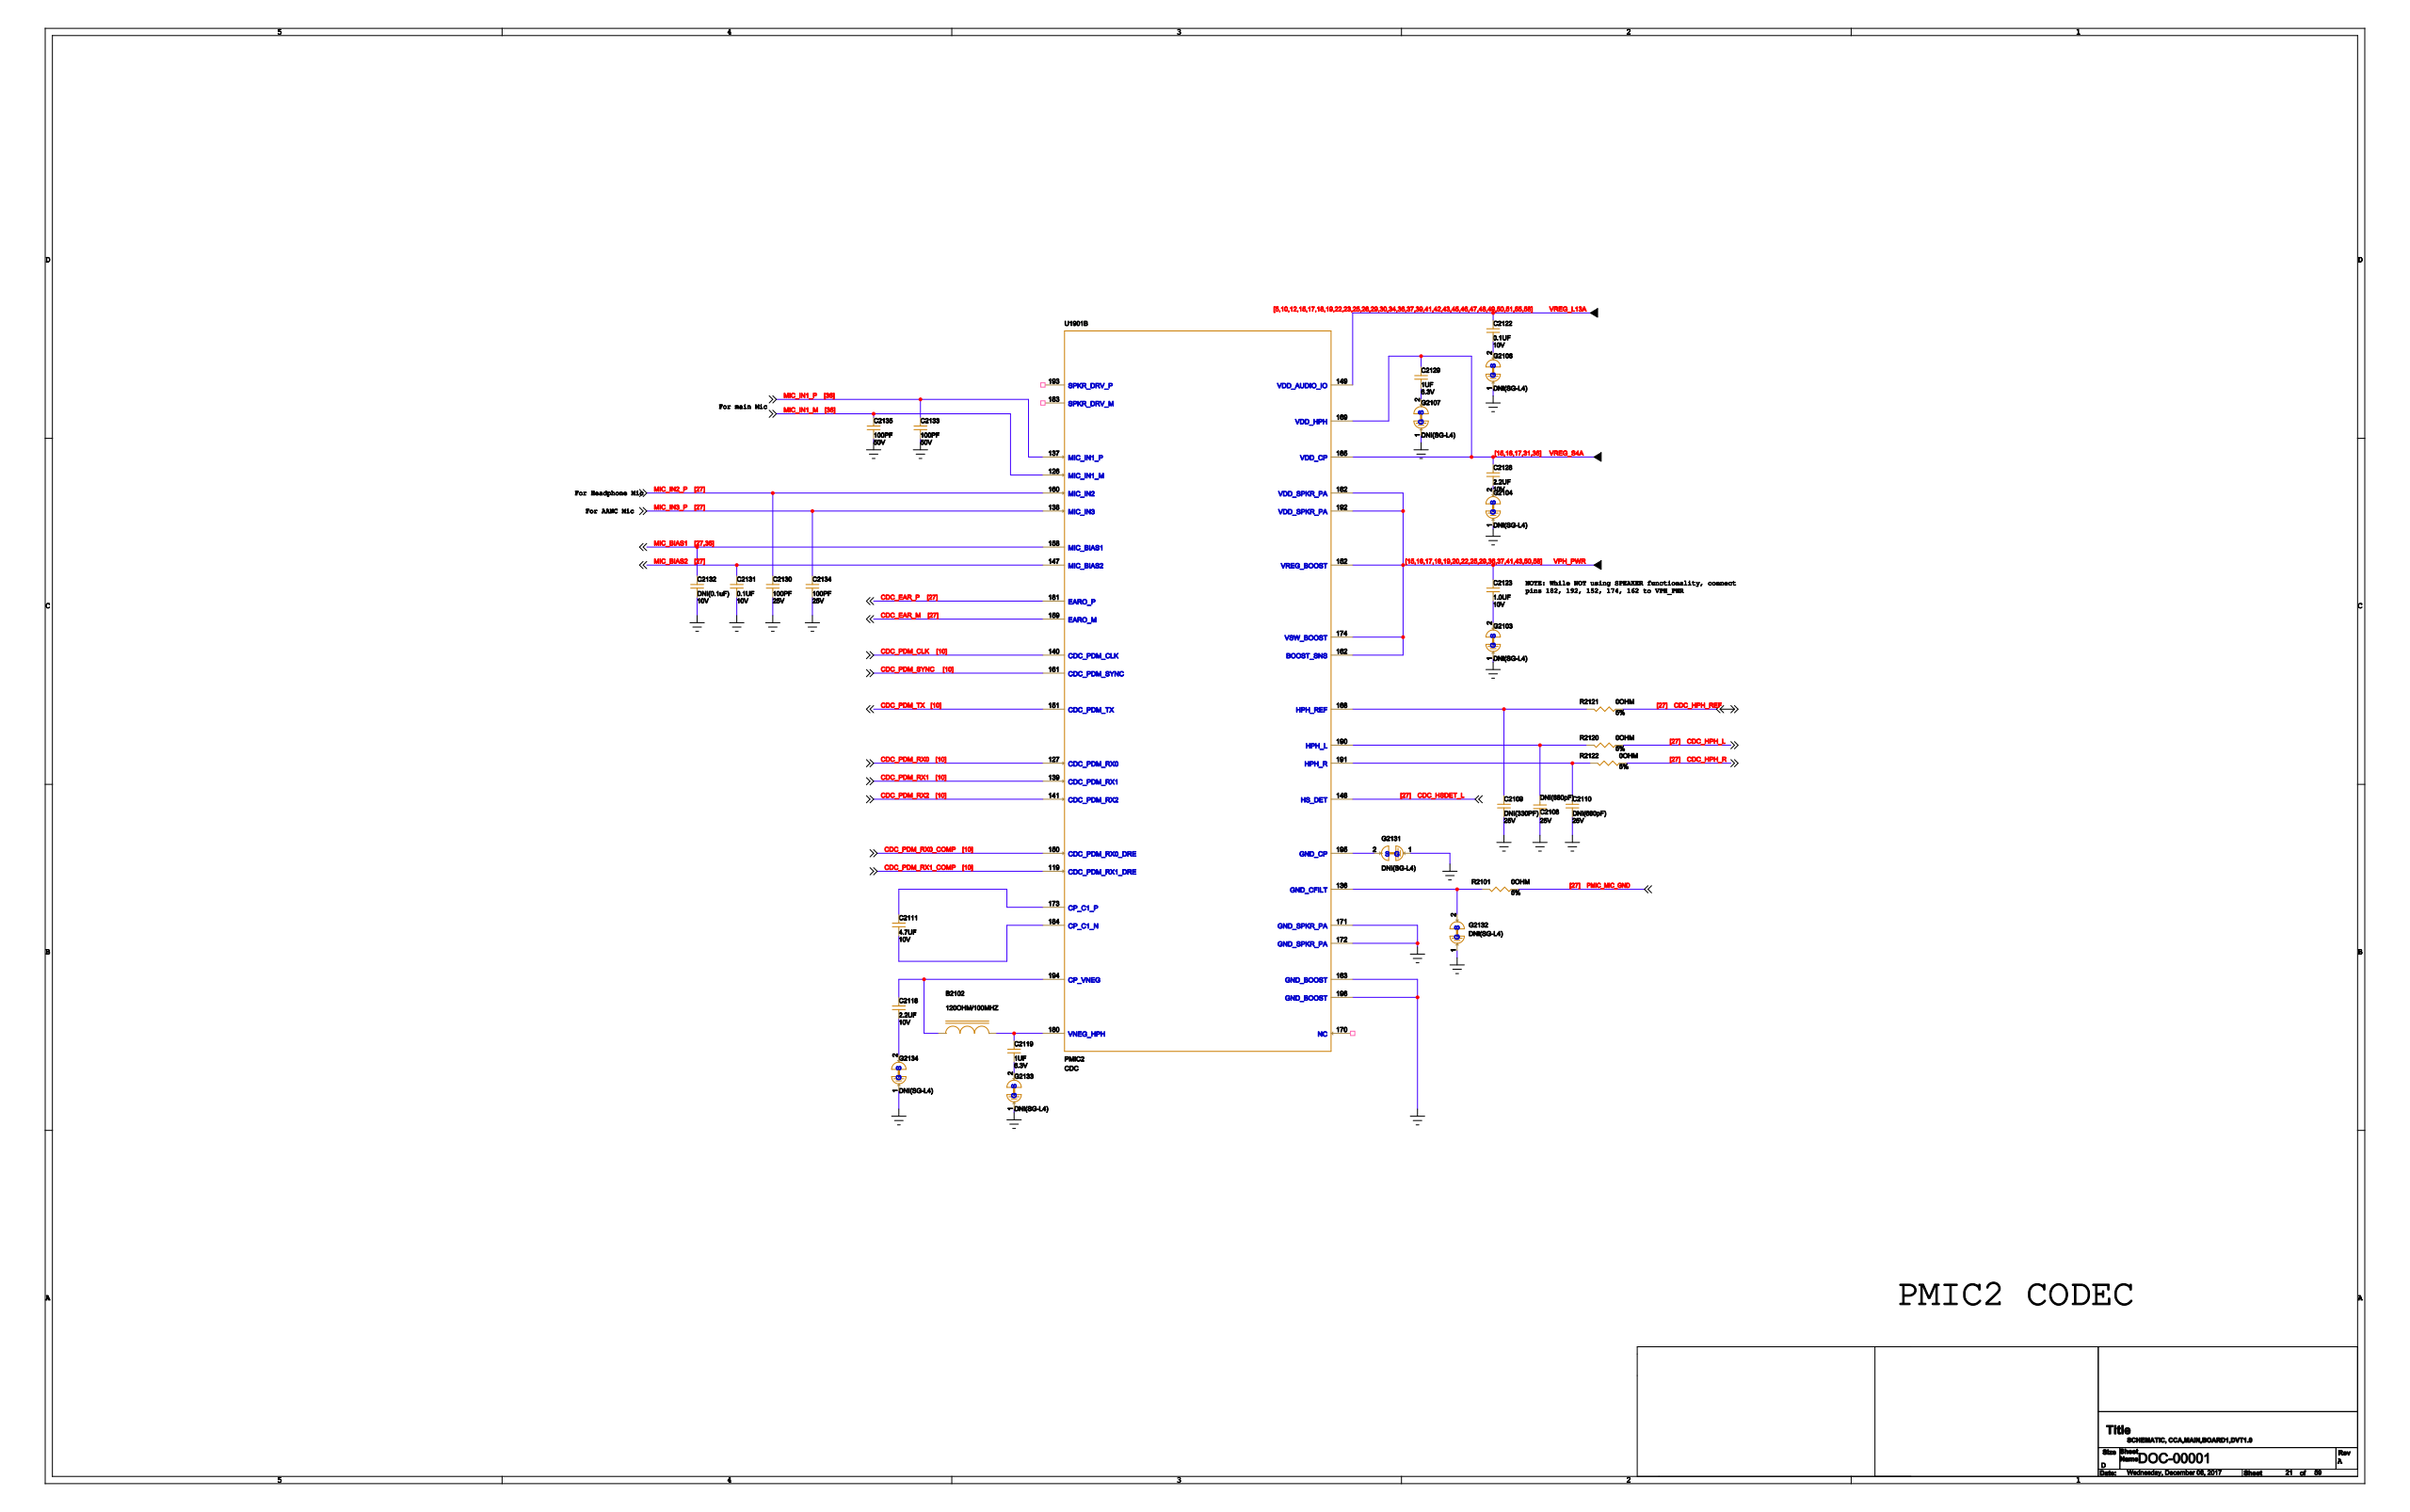Circuit board | KiCad | 1657 parts | 1365 nets | one sheet of the schematic
Parts on this sheet (reference | value | footprint):
B2102
C2108
C2109
C2110
C2111
C2118
C2119
C2122
C2123
C2128
C2129
C2130
C2131
C2132
C2133
C2134
C2135
G2103
G2104
G2106
G2107
G2131
G2132
G2133
G2134
R2101
R2120
R2121
R2122
U1901
Nets of these parts (net: part-pin ...):
CDC_EAR_P: U1901-181
GND: C2108-1 C2109-2 C2110-2 C2130-2 C2131-2 C2132-2 C2133-2 C2134-2 C2135-2 G2103-1 G2104-1 G2106-1 G2107-1 G2131-1 G2132-1 G2133-1 G2134-1 U1901-163 U1901-171 U1901-172 U1901-196
VREG_L13A: C2122-1 U1901-149
VPH_PWR: C2123-1 U1901-2 U1901-17 U1901-21 U1901-39 U1901-152 U1901-162 U1901-174 U1901-182 U1901-192
MIC_BIAS1: C2132-1 U1901-158
N22309812: G2131-2 U1901-195
N22309894: C2118-2 G2134-2
MIC_IN1_M: C2135-1 U1901-126
MIC_IN1_P: C2133-1 U1901-137
N22309718: G2132-2 R2101-1 U1901-136
CDC_HPH_R: R2122-2
CDC_EAR_M: U1901-159
CDC_HPH_L: R2120-2
CDC_HPH_REF: R2121-2
VREG_S4A: C2128-1 C2129-1 U1901-169 U1901-185
CDC_HSDET_L: U1901-148
N22309806: C2129-2 G2107-2
N22309778: C2128-2 G2104-2
CDC_PDM_RX1: U1901-139
CDC_PDM_TX: U1901-151
CDC_PDM_RX0: U1901-127
CDC_PDM_CLK: U1901-140
CDC_PDM_SYNC: U1901-161
CDC_PDM_RX2: U1901-141
N22309760: C2123-2 G2103-2
N22309788: C2122-2 G2106-2
N22309892: C2119-2 G2133-2
MIC_IN2_P: C2130-1 U1901-160
N22309740: C2108-2 R2120-1 U1901-190
MIC_IN3_P: C2134-1 U1901-138
N22309724: C2109-1 R2121-1 U1901-168
PMIC_MIC_GND: R2101-2
N22309860: B2102-1 C2118-1 U1901-194
N22309864: B2102-2 C2119-1 U1901-180
MIC_BIAS2: C2131-1 U1901-147
N22309876: C2111-1 U1901-173
N22309884: C2111-2 U1901-184
N22309734: C2110-1 R2122-1 U1901-191